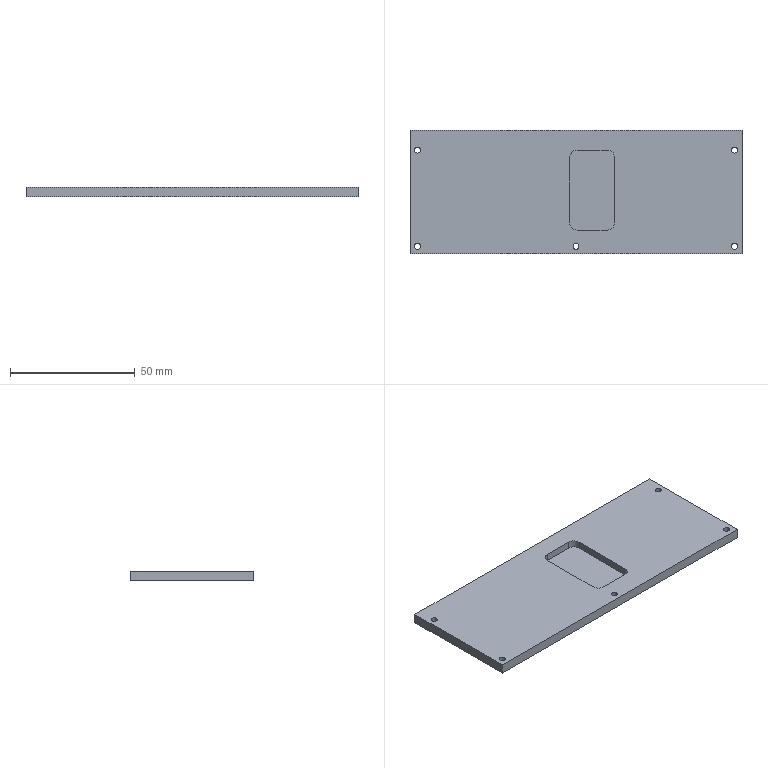Part | 1 solid | 48 faces | box 133 x 49.5 x 4 mm | volume 24425 mm3 | cylinder 28 | plane 16 | cone 4 | commonest cylinder face diameters 2.4 x10 4 x10 1.6 x4 6 x4
STEP:
#1=CARTESIAN_POINT('',(31.5,19.55,-2.8));
#2=VERTEX_POINT('',#1);
#3=CARTESIAN_POINT('',(31.5,19.55,-1.2));
#4=VERTEX_POINT('',#3);
#5=CARTESIAN_POINT('',(31.5,19.55,-2.));
#6=DIRECTION('',(0.,1.,0.));
#7=DIRECTION('',(0.,0.,1.));
#8=AXIS2_PLACEMENT_3D('',#5,#6,#7);
#9=CIRCLE('',#8,0.8);
#10=EDGE_CURVE('',#2,#4,#9,.T.);
#11=ORIENTED_EDGE('',*,*,#10,.F.);
#12=CARTESIAN_POINT('',(31.5,24.75,-2.8));
#13=VERTEX_POINT('',#12);
#14=CARTESIAN_POINT('',(31.5,24.75,-2.8));
#15=DIRECTION('',(0.,1.,0.));
#16=VECTOR('',#15,1000.);
#17=LINE('',#14,#16);
#18=EDGE_CURVE('',#2,#13,#17,.T.);
#19=ORIENTED_EDGE('',*,*,#18,.T.);
#20=CARTESIAN_POINT('',(31.5,24.75,-1.2));
#21=VERTEX_POINT('',#20);
#22=CARTESIAN_POINT('',(31.5,24.75,-2.));
#23=DIRECTION('',(0.,1.,0.));
#24=DIRECTION('',(0.,0.,1.));
#25=AXIS2_PLACEMENT_3D('',#22,#23,#24);
#26=CIRCLE('',#25,0.8);
#27=EDGE_CURVE('',#13,#21,#26,.T.);
#28=ORIENTED_EDGE('',*,*,#27,.T.);
#29=CARTESIAN_POINT('',(31.5,24.75,-1.2));
#30=DIRECTION('',(0.,1.,0.));
#31=VECTOR('',#30,1000.);
#32=LINE('',#29,#31);
#33=EDGE_CURVE('',#4,#21,#32,.T.);
#34=ORIENTED_EDGE('',*,*,#33,.F.);
#35=EDGE_LOOP('',(#11,#19,#28,#34));
#36=FACE_BOUND('',#35,.T.);
#37=CARTESIAN_POINT('',(31.5,24.75,-2.));
#38=DIRECTION('',(0.,1.,0.));
#39=DIRECTION('',(0.,0.,-1.));
#40=AXIS2_PLACEMENT_3D('',#37,#38,#39);
#41=CYLINDRICAL_SURFACE('',#40,0.8);
#42=ADVANCED_FACE('',(#36),#41,.F.);
#43=CARTESIAN_POINT('',(31.5,19.069,-2.));
#44=VERTEX_POINT('',#43);
#45=CARTESIAN_POINT('',(31.5,19.55,-1.2));
#46=DIRECTION('',(0.,0.515,0.8572));
#47=VECTOR('',#46,1000.);
#48=LINE('',#45,#47);
#49=EDGE_CURVE('',#44,#4,#48,.T.);
#50=ORIENTED_EDGE('',*,*,#49,.F.);
#51=CARTESIAN_POINT('',(31.5,19.55,-2.8));
#52=DIRECTION('',(0.,0.515,-0.8572));
#53=VECTOR('',#52,1000.);
#54=LINE('',#51,#53);
#55=EDGE_CURVE('',#44,#2,#54,.T.);
#56=ORIENTED_EDGE('',*,*,#55,.T.);
#57=ORIENTED_EDGE('',*,*,#10,.T.);
#58=EDGE_LOOP('',(#50,#56,#57));
#59=FACE_BOUND('',#58,.T.);
#60=CARTESIAN_POINT('',(31.5,19.55,-2.));
#61=DIRECTION('',(0.,1.,0.));
#62=DIRECTION('',(0.,0.,-1.));
#63=AXIS2_PLACEMENT_3D('',#60,#61,#62);
#64=CONICAL_SURFACE('',#63,0.8,1.03);
#65=ADVANCED_FACE('',(#59),#64,.F.);
#66=CARTESIAN_POINT('',(-31.5,19.55,-2.8));
#67=VERTEX_POINT('',#66);
#68=CARTESIAN_POINT('',(-31.5,19.55,-1.2));
#69=VERTEX_POINT('',#68);
#70=CARTESIAN_POINT('',(-31.5,19.55,-2.));
#71=DIRECTION('',(0.,1.,0.));
#72=DIRECTION('',(0.,0.,1.));
#73=AXIS2_PLACEMENT_3D('',#70,#71,#72);
#74=CIRCLE('',#73,0.8);
#75=EDGE_CURVE('',#67,#69,#74,.T.);
#76=ORIENTED_EDGE('',*,*,#75,.F.);
#77=CARTESIAN_POINT('',(-31.5,24.75,-2.8));
#78=VERTEX_POINT('',#77);
#79=CARTESIAN_POINT('',(-31.5,24.75,-2.8));
#80=DIRECTION('',(0.,1.,0.));
#81=VECTOR('',#80,1000.);
#82=LINE('',#79,#81);
#83=EDGE_CURVE('',#67,#78,#82,.T.);
#84=ORIENTED_EDGE('',*,*,#83,.T.);
#85=CARTESIAN_POINT('',(-31.5,24.75,-1.2));
#86=VERTEX_POINT('',#85);
#87=CARTESIAN_POINT('',(-31.5,24.75,-2.));
#88=DIRECTION('',(0.,1.,0.));
#89=DIRECTION('',(0.,0.,1.));
#90=AXIS2_PLACEMENT_3D('',#87,#88,#89);
#91=CIRCLE('',#90,0.8);
#92=EDGE_CURVE('',#78,#86,#91,.T.);
#93=ORIENTED_EDGE('',*,*,#92,.T.);
#94=CARTESIAN_POINT('',(-31.5,24.75,-1.2));
#95=DIRECTION('',(0.,1.,0.));
#96=VECTOR('',#95,1000.);
#97=LINE('',#94,#96);
#98=EDGE_CURVE('',#69,#86,#97,.T.);
#99=ORIENTED_EDGE('',*,*,#98,.F.);
#100=EDGE_LOOP('',(#76,#84,#93,#99));
#101=FACE_BOUND('',#100,.T.);
#102=CARTESIAN_POINT('',(-31.5,24.75,-2.));
#103=DIRECTION('',(0.,1.,0.));
#104=DIRECTION('',(0.,0.,-1.));
#105=AXIS2_PLACEMENT_3D('',#102,#103,#104);
#106=CYLINDRICAL_SURFACE('',#105,0.8);
#107=ADVANCED_FACE('',(#101),#106,.F.);
#108=CARTESIAN_POINT('',(-31.5,19.069,-2.));
#109=VERTEX_POINT('',#108);
#110=CARTESIAN_POINT('',(-31.5,19.55,-1.2));
#111=DIRECTION('',(0.,0.515,0.8572));
#112=VECTOR('',#111,1000.);
#113=LINE('',#110,#112);
#114=EDGE_CURVE('',#109,#69,#113,.T.);
#115=ORIENTED_EDGE('',*,*,#114,.F.);
#116=CARTESIAN_POINT('',(-31.5,19.55,-2.8));
#117=DIRECTION('',(0.,0.515,-0.8572));
#118=VECTOR('',#117,1000.);
#119=LINE('',#116,#118);
#120=EDGE_CURVE('',#109,#67,#119,.T.);
#121=ORIENTED_EDGE('',*,*,#120,.T.);
#122=ORIENTED_EDGE('',*,*,#75,.T.);
#123=EDGE_LOOP('',(#115,#121,#122));
#124=FACE_BOUND('',#123,.T.);
#125=CARTESIAN_POINT('',(-31.5,19.55,-2.));
#126=DIRECTION('',(0.,1.,0.));
#127=DIRECTION('',(0.,0.,-1.));
#128=AXIS2_PLACEMENT_3D('',#125,#126,#127);
#129=CONICAL_SURFACE('',#128,0.8,1.03);
#130=ADVANCED_FACE('',(#124),#129,.F.);
#131=CARTESIAN_POINT('',(-61.5,16.75,-1.7));
#132=VERTEX_POINT('',#131);
#133=CARTESIAN_POINT('',(-65.5,16.75,-1.7));
#134=VERTEX_POINT('',#133);
#135=CARTESIAN_POINT('',(-63.5,16.75,-1.7));
#136=DIRECTION('',(0.,0.,-1.));
#137=DIRECTION('',(-1.,0.,0.));
#138=AXIS2_PLACEMENT_3D('',#135,#136,#137);
#139=CIRCLE('',#138,2.);
#140=EDGE_CURVE('',#132,#134,#139,.T.);
#141=ORIENTED_EDGE('',*,*,#140,.F.);
#142=CARTESIAN_POINT('',(-61.5,16.75,-4.));
#143=VERTEX_POINT('',#142);
#144=CARTESIAN_POINT('',(-61.5,16.75,-4.));
#145=DIRECTION('',(0.,0.,-1.));
#146=VECTOR('',#145,1000.);
#147=LINE('',#144,#146);
#148=EDGE_CURVE('',#132,#143,#147,.T.);
#149=ORIENTED_EDGE('',*,*,#148,.T.);
#150=CARTESIAN_POINT('',(-65.5,16.75,-4.));
#151=VERTEX_POINT('',#150);
#152=CARTESIAN_POINT('',(-63.5,16.75,-4.));
#153=DIRECTION('',(0.,0.,-1.));
#154=DIRECTION('',(-1.,0.,0.));
#155=AXIS2_PLACEMENT_3D('',#152,#153,#154);
#156=CIRCLE('',#155,2.);
#157=EDGE_CURVE('',#143,#151,#156,.T.);
#158=ORIENTED_EDGE('',*,*,#157,.T.);
#159=CARTESIAN_POINT('',(-65.5,16.75,-4.));
#160=DIRECTION('',(0.,0.,-1.));
#161=VECTOR('',#160,1000.);
#162=LINE('',#159,#161);
#163=EDGE_CURVE('',#134,#151,#162,.T.);
#164=ORIENTED_EDGE('',*,*,#163,.F.);
#165=EDGE_LOOP('',(#141,#149,#158,#164));
#166=FACE_BOUND('',#165,.T.);
#167=CARTESIAN_POINT('',(-63.5,16.75,-4.));
#168=DIRECTION('',(0.,0.,-1.));
#169=DIRECTION('',(1.,0.,0.));
#170=AXIS2_PLACEMENT_3D('',#167,#168,#169);
#171=CYLINDRICAL_SURFACE('',#170,2.);
#172=ADVANCED_FACE('',(#166),#171,.F.);
#173=CARTESIAN_POINT('',(-64.7,16.75,0.));
#174=VERTEX_POINT('',#173);
#175=CARTESIAN_POINT('',(-62.3,16.75,0.));
#176=VERTEX_POINT('',#175);
#177=CARTESIAN_POINT('',(-63.5,16.75,0.));
#178=DIRECTION('',(0.,0.,1.));
#179=DIRECTION('',(1.,0.,0.));
#180=AXIS2_PLACEMENT_3D('',#177,#178,#179);
#181=CIRCLE('',#180,1.2);
#182=EDGE_CURVE('',#174,#176,#181,.T.);
#183=ORIENTED_EDGE('',*,*,#182,.T.);
#184=CARTESIAN_POINT('',(-62.3,16.75,-1.7));
#185=VERTEX_POINT('',#184);
#186=CARTESIAN_POINT('',(-62.3,16.75,-4.));
#187=DIRECTION('',(0.,0.,-1.));
#188=VECTOR('',#187,1000.);
#189=LINE('',#186,#188);
#190=EDGE_CURVE('',#176,#185,#189,.T.);
#191=ORIENTED_EDGE('',*,*,#190,.T.);
#192=CARTESIAN_POINT('',(-64.7,16.75,-1.7));
#193=VERTEX_POINT('',#192);
#194=CARTESIAN_POINT('',(-63.5,16.75,-1.7));
#195=DIRECTION('',(0.,0.,-1.));
#196=DIRECTION('',(-1.,0.,0.));
#197=AXIS2_PLACEMENT_3D('',#194,#195,#196);
#198=CIRCLE('',#197,1.2);
#199=EDGE_CURVE('',#185,#193,#198,.T.);
#200=ORIENTED_EDGE('',*,*,#199,.T.);
#201=CARTESIAN_POINT('',(-64.7,16.75,-4.));
#202=DIRECTION('',(0.,0.,-1.));
#203=VECTOR('',#202,1000.);
#204=LINE('',#201,#203);
#205=EDGE_CURVE('',#174,#193,#204,.T.);
#206=ORIENTED_EDGE('',*,*,#205,.F.);
#207=EDGE_LOOP('',(#183,#191,#200,#206));
#208=FACE_BOUND('',#207,.T.);
#209=CARTESIAN_POINT('',(-63.5,16.75,-4.));
#210=DIRECTION('',(0.,0.,-1.));
#211=DIRECTION('',(1.,0.,0.));
#212=AXIS2_PLACEMENT_3D('',#209,#210,#211);
#213=CYLINDRICAL_SURFACE('',#212,1.2);
#214=ADVANCED_FACE('',(#208),#213,.F.);
#215=CARTESIAN_POINT('',(-61.5,-21.75,-1.7));
#216=VERTEX_POINT('',#215);
#217=CARTESIAN_POINT('',(-65.5,-21.75,-1.7));
#218=VERTEX_POINT('',#217);
#219=CARTESIAN_POINT('',(-63.5,-21.75,-1.7));
#220=DIRECTION('',(0.,0.,-1.));
#221=DIRECTION('',(-1.,0.,0.));
#222=AXIS2_PLACEMENT_3D('',#219,#220,#221);
#223=CIRCLE('',#222,2.);
#224=EDGE_CURVE('',#216,#218,#223,.T.);
#225=ORIENTED_EDGE('',*,*,#224,.F.);
#226=CARTESIAN_POINT('',(-61.5,-21.75,-4.));
#227=VERTEX_POINT('',#226);
#228=CARTESIAN_POINT('',(-61.5,-21.75,-4.));
#229=DIRECTION('',(0.,0.,-1.));
#230=VECTOR('',#229,1000.);
#231=LINE('',#228,#230);
#232=EDGE_CURVE('',#216,#227,#231,.T.);
#233=ORIENTED_EDGE('',*,*,#232,.T.);
#234=CARTESIAN_POINT('',(-65.5,-21.75,-4.));
#235=VERTEX_POINT('',#234);
#236=CARTESIAN_POINT('',(-63.5,-21.75,-4.));
#237=DIRECTION('',(0.,0.,-1.));
#238=DIRECTION('',(-1.,0.,0.));
#239=AXIS2_PLACEMENT_3D('',#236,#237,#238);
#240=CIRCLE('',#239,2.);
#241=EDGE_CURVE('',#227,#235,#240,.T.);
#242=ORIENTED_EDGE('',*,*,#241,.T.);
#243=CARTESIAN_POINT('',(-65.5,-21.75,-4.));
#244=DIRECTION('',(0.,0.,-1.));
#245=VECTOR('',#244,1000.);
#246=LINE('',#243,#245);
#247=EDGE_CURVE('',#218,#235,#246,.T.);
#248=ORIENTED_EDGE('',*,*,#247,.F.);
#249=EDGE_LOOP('',(#225,#233,#242,#248));
#250=FACE_BOUND('',#249,.T.);
#251=CARTESIAN_POINT('',(-63.5,-21.75,-4.));
#252=DIRECTION('',(0.,0.,-1.));
#253=DIRECTION('',(1.,0.,0.));
#254=AXIS2_PLACEMENT_3D('',#251,#252,#253);
#255=CYLINDRICAL_SURFACE('',#254,2.);
#256=ADVANCED_FACE('',(#250),#255,.F.);
#257=CARTESIAN_POINT('',(-64.7,-21.75,0.));
#258=VERTEX_POINT('',#257);
#259=CARTESIAN_POINT('',(-62.3,-21.75,0.));
#260=VERTEX_POINT('',#259);
#261=CARTESIAN_POINT('',(-63.5,-21.75,0.));
#262=DIRECTION('',(0.,0.,1.));
#263=DIRECTION('',(1.,0.,0.));
#264=AXIS2_PLACEMENT_3D('',#261,#262,#263);
#265=CIRCLE('',#264,1.2);
#266=EDGE_CURVE('',#258,#260,#265,.T.);
#267=ORIENTED_EDGE('',*,*,#266,.T.);
#268=CARTESIAN_POINT('',(-62.3,-21.75,-1.7));
#269=VERTEX_POINT('',#268);
#270=CARTESIAN_POINT('',(-62.3,-21.75,-4.));
#271=DIRECTION('',(0.,0.,-1.));
#272=VECTOR('',#271,1000.);
#273=LINE('',#270,#272);
#274=EDGE_CURVE('',#260,#269,#273,.T.);
#275=ORIENTED_EDGE('',*,*,#274,.T.);
#276=CARTESIAN_POINT('',(-64.7,-21.75,-1.7));
#277=VERTEX_POINT('',#276);
#278=CARTESIAN_POINT('',(-63.5,-21.75,-1.7));
#279=DIRECTION('',(0.,0.,-1.));
#280=DIRECTION('',(-1.,0.,0.));
#281=AXIS2_PLACEMENT_3D('',#278,#279,#280);
#282=CIRCLE('',#281,1.2);
#283=EDGE_CURVE('',#269,#277,#282,.T.);
#284=ORIENTED_EDGE('',*,*,#283,.T.);
#285=CARTESIAN_POINT('',(-64.7,-21.75,-4.));
#286=DIRECTION('',(0.,0.,-1.));
#287=VECTOR('',#286,1000.);
#288=LINE('',#285,#287);
#289=EDGE_CURVE('',#258,#277,#288,.T.);
#290=ORIENTED_EDGE('',*,*,#289,.F.);
#291=EDGE_LOOP('',(#267,#275,#284,#290));
#292=FACE_BOUND('',#291,.T.);
#293=CARTESIAN_POINT('',(-63.5,-21.75,-4.));
#294=DIRECTION('',(0.,0.,-1.));
#295=DIRECTION('',(1.,0.,0.));
#296=AXIS2_PLACEMENT_3D('',#293,#294,#295);
#297=CYLINDRICAL_SURFACE('',#296,1.2);
#298=ADVANCED_FACE('',(#292),#297,.F.);
#299=CARTESIAN_POINT('',(2.,-21.75,-1.7));
#300=VERTEX_POINT('',#299);
#301=CARTESIAN_POINT('',(-2.,-21.75,-1.7));
#302=VERTEX_POINT('',#301);
#303=CARTESIAN_POINT('',(0.,-21.75,-1.7));
#304=DIRECTION('',(0.,0.,-1.));
#305=DIRECTION('',(-1.,0.,0.));
#306=AXIS2_PLACEMENT_3D('',#303,#304,#305);
#307=CIRCLE('',#306,2.);
#308=EDGE_CURVE('',#300,#302,#307,.T.);
#309=ORIENTED_EDGE('',*,*,#308,.F.);
#310=CARTESIAN_POINT('',(2.,-21.75,-4.));
#311=VERTEX_POINT('',#310);
#312=CARTESIAN_POINT('',(2.,-21.75,-4.));
#313=DIRECTION('',(0.,0.,-1.));
#314=VECTOR('',#313,1000.);
#315=LINE('',#312,#314);
#316=EDGE_CURVE('',#300,#311,#315,.T.);
#317=ORIENTED_EDGE('',*,*,#316,.T.);
#318=CARTESIAN_POINT('',(-2.,-21.75,-4.));
#319=VERTEX_POINT('',#318);
#320=CARTESIAN_POINT('',(0.,-21.75,-4.));
#321=DIRECTION('',(0.,0.,-1.));
#322=DIRECTION('',(-1.,0.,0.));
#323=AXIS2_PLACEMENT_3D('',#320,#321,#322);
#324=CIRCLE('',#323,2.);
#325=EDGE_CURVE('',#311,#319,#324,.T.);
#326=ORIENTED_EDGE('',*,*,#325,.T.);
#327=CARTESIAN_POINT('',(-2.,-21.75,-4.));
#328=DIRECTION('',(0.,0.,-1.));
#329=VECTOR('',#328,1000.);
#330=LINE('',#327,#329);
#331=EDGE_CURVE('',#302,#319,#330,.T.);
#332=ORIENTED_EDGE('',*,*,#331,.F.);
#333=EDGE_LOOP('',(#309,#317,#326,#332));
#334=FACE_BOUND('',#333,.T.);
#335=CARTESIAN_POINT('',(0.,-21.75,-4.));
#336=DIRECTION('',(0.,0.,-1.));
#337=DIRECTION('',(1.,0.,0.));
#338=AXIS2_PLACEMENT_3D('',#335,#336,#337);
#339=CYLINDRICAL_SURFACE('',#338,2.);
#340=ADVANCED_FACE('',(#334),#339,.F.);
#341=CARTESIAN_POINT('',(-1.2,-21.75,0.));
#342=VERTEX_POINT('',#341);
#343=CARTESIAN_POINT('',(1.2,-21.75,0.));
#344=VERTEX_POINT('',#343);
#345=CARTESIAN_POINT('',(0.,-21.75,0.));
#346=DIRECTION('',(0.,0.,1.));
#347=DIRECTION('',(1.,0.,0.));
#348=AXIS2_PLACEMENT_3D('',#345,#346,#347);
#349=CIRCLE('',#348,1.2);
#350=EDGE_CURVE('',#342,#344,#349,.T.);
#351=ORIENTED_EDGE('',*,*,#350,.T.);
#352=CARTESIAN_POINT('',(1.2,-21.75,-1.7));
#353=VERTEX_POINT('',#352);
#354=CARTESIAN_POINT('',(1.2,-21.75,-4.));
#355=DIRECTION('',(0.,0.,-1.));
#356=VECTOR('',#355,1000.);
#357=LINE('',#354,#356);
#358=EDGE_CURVE('',#344,#353,#357,.T.);
#359=ORIENTED_EDGE('',*,*,#358,.T.);
#360=CARTESIAN_POINT('',(-1.2,-21.75,-1.7));
#361=VERTEX_POINT('',#360);
#362=CARTESIAN_POINT('',(0.,-21.75,-1.7));
#363=DIRECTION('',(0.,0.,-1.));
#364=DIRECTION('',(-1.,0.,0.));
#365=AXIS2_PLACEMENT_3D('',#362,#363,#364);
#366=CIRCLE('',#365,1.2);
#367=EDGE_CURVE('',#353,#361,#366,.T.);
#368=ORIENTED_EDGE('',*,*,#367,.T.);
#369=CARTESIAN_POINT('',(-1.2,-21.75,-4.));
#370=DIRECTION('',(0.,0.,-1.));
#371=VECTOR('',#370,1000.);
#372=LINE('',#369,#371);
#373=EDGE_CURVE('',#342,#361,#372,.T.);
#374=ORIENTED_EDGE('',*,*,#373,.F.);
#375=EDGE_LOOP('',(#351,#359,#368,#374));
#376=FACE_BOUND('',#375,.T.);
#377=CARTESIAN_POINT('',(0.,-21.75,-4.));
#378=DIRECTION('',(0.,0.,-1.));
#379=DIRECTION('',(1.,0.,0.));
#380=AXIS2_PLACEMENT_3D('',#377,#378,#379);
#381=CYLINDRICAL_SURFACE('',#380,1.2);
#382=ADVANCED_FACE('',(#376),#381,.F.);
#383=CARTESIAN_POINT('',(65.5,-21.75,-1.7));
#384=VERTEX_POINT('',#383);
#385=CARTESIAN_POINT('',(61.5,-21.75,-1.7));
#386=VERTEX_POINT('',#385);
#387=CARTESIAN_POINT('',(63.5,-21.75,-1.7));
#388=DIRECTION('',(0.,0.,-1.));
#389=DIRECTION('',(-1.,0.,0.));
#390=AXIS2_PLACEMENT_3D('',#387,#388,#389);
#391=CIRCLE('',#390,2.);
#392=EDGE_CURVE('',#384,#386,#391,.T.);
#393=ORIENTED_EDGE('',*,*,#392,.F.);
#394=CARTESIAN_POINT('',(65.5,-21.75,-4.));
#395=VERTEX_POINT('',#394);
#396=CARTESIAN_POINT('',(65.5,-21.75,-4.));
#397=DIRECTION('',(0.,0.,-1.));
#398=VECTOR('',#397,1000.);
#399=LINE('',#396,#398);
#400=EDGE_CURVE('',#384,#395,#399,.T.);
#401=ORIENTED_EDGE('',*,*,#400,.T.);
#402=CARTESIAN_POINT('',(61.5,-21.75,-4.));
#403=VERTEX_POINT('',#402);
#404=CARTESIAN_POINT('',(63.5,-21.75,-4.));
#405=DIRECTION('',(0.,0.,-1.));
#406=DIRECTION('',(-1.,0.,0.));
#407=AXIS2_PLACEMENT_3D('',#404,#405,#406);
#408=CIRCLE('',#407,2.);
#409=EDGE_CURVE('',#395,#403,#408,.T.);
#410=ORIENTED_EDGE('',*,*,#409,.T.);
#411=CARTESIAN_POINT('',(61.5,-21.75,-4.));
#412=DIRECTION('',(0.,0.,-1.));
#413=VECTOR('',#412,1000.);
#414=LINE('',#411,#413);
#415=EDGE_CURVE('',#386,#403,#414,.T.);
#416=ORIENTED_EDGE('',*,*,#415,.F.);
#417=EDGE_LOOP('',(#393,#401,#410,#416));
#418=FACE_BOUND('',#417,.T.);
#419=CARTESIAN_POINT('',(63.5,-21.75,-4.));
#420=DIRECTION('',(0.,0.,-1.));
#421=DIRECTION('',(1.,0.,0.));
#422=AXIS2_PLACEMENT_3D('',#419,#420,#421);
#423=CYLINDRICAL_SURFACE('',#422,2.);
#424=ADVANCED_FACE('',(#418),#423,.F.);
#425=CARTESIAN_POINT('',(62.3,-21.75,0.));
#426=VERTEX_POINT('',#425);
#427=CARTESIAN_POINT('',(64.7,-21.75,0.));
#428=VERTEX_POINT('',#427);
#429=CARTESIAN_POINT('',(63.5,-21.75,0.));
#430=DIRECTION('',(0.,0.,1.));
#431=DIRECTION('',(1.,0.,0.));
#432=AXIS2_PLACEMENT_3D('',#429,#430,#431);
#433=CIRCLE('',#432,1.2);
#434=EDGE_CURVE('',#426,#428,#433,.T.);
#435=ORIENTED_EDGE('',*,*,#434,.T.);
#436=CARTESIAN_POINT('',(64.7,-21.75,-1.7));
#437=VERTEX_POINT('',#436);
#438=CARTESIAN_POINT('',(64.7,-21.75,-4.));
#439=DIRECTION('',(0.,0.,-1.));
#440=VECTOR('',#439,1000.);
#441=LINE('',#438,#440);
#442=EDGE_CURVE('',#428,#437,#441,.T.);
#443=ORIENTED_EDGE('',*,*,#442,.T.);
#444=CARTESIAN_POINT('',(62.3,-21.75,-1.7));
#445=VERTEX_POINT('',#444);
#446=CARTESIAN_POINT('',(63.5,-21.75,-1.7));
#447=DIRECTION('',(0.,0.,-1.));
#448=DIRECTION('',(-1.,0.,0.));
#449=AXIS2_PLACEMENT_3D('',#446,#447,#448);
#450=CIRCLE('',#449,1.2);
#451=EDGE_CURVE('',#437,#445,#450,.T.);
#452=ORIENTED_EDGE('',*,*,#451,.T.);
#453=CARTESIAN_POINT('',(62.3,-21.75,-4.));
#454=DIRECTION('',(0.,0.,-1.));
#455=VECTOR('',#454,1000.);
#456=LINE('',#453,#455);
#457=EDGE_CURVE('',#426,#445,#456,.T.);
#458=ORIENTED_EDGE('',*,*,#457,.F.);
#459=EDGE_LOOP('',(#435,#443,#452,#458));
#460=FACE_BOUND('',#459,.T.);
#461=CARTESIAN_POINT('',(63.5,-21.75,-4.));
#462=DIRECTION('',(0.,0.,-1.));
#463=DIRECTION('',(1.,0.,0.));
#464=AXIS2_PLACEMENT_3D('',#461,#462,#463);
#465=CYLINDRICAL_SURFACE('',#464,1.2);
#466=ADVANCED_FACE('',(#460),#465,.F.);
#467=CARTESIAN_POINT('',(65.5,16.75,-1.7));
#468=VERTEX_POINT('',#467);
#469=CARTESIAN_POINT('',(61.5,16.75,-1.7));
#470=VERTEX_POINT('',#469);
#471=CARTESIAN_POINT('',(63.5,16.75,-1.7));
#472=DIRECTION('',(0.,0.,-1.));
#473=DIRECTION('',(-1.,0.,0.));
#474=AXIS2_PLACEMENT_3D('',#471,#472,#473);
#475=CIRCLE('',#474,2.);
#476=EDGE_CURVE('',#468,#470,#475,.T.);
#477=ORIENTED_EDGE('',*,*,#476,.F.);
#478=CARTESIAN_POINT('',(65.5,16.75,-4.));
#479=VERTEX_POINT('',#478);
#480=CARTESIAN_POINT('',(65.5,16.75,-4.));
#481=DIRECTION('',(0.,0.,-1.));
#482=VECTOR('',#481,1000.);
#483=LINE('',#480,#482);
#484=EDGE_CURVE('',#468,#479,#483,.T.);
#485=ORIENTED_EDGE('',*,*,#484,.T.);
#486=CARTESIAN_POINT('',(61.5,16.75,-4.));
#487=VERTEX_POINT('',#486);
#488=CARTESIAN_POINT('',(63.5,16.75,-4.));
#489=DIRECTION('',(0.,0.,-1.));
#490=DIRECTION('',(-1.,0.,0.));
#491=AXIS2_PLACEMENT_3D('',#488,#489,#490);
#492=CIRCLE('',#491,2.);
#493=EDGE_CURVE('',#479,#487,#492,.T.);
#494=ORIENTED_EDGE('',*,*,#493,.T.);
#495=CARTESIAN_POINT('',(61.5,16.75,-4.));
#496=DIRECTION('',(0.,0.,-1.));
#497=VECTOR('',#496,1000.);
#498=LINE('',#495,#497);
#499=EDGE_CURVE('',#470,#487,#498,.T.);
#500=ORIENTED_EDGE('',*,*,#499,.F.);
#501=EDGE_LOOP('',(#477,#485,#494,#500));
#502=FACE_BOUND('',#501,.T.);
#503=CARTESIAN_POINT('',(63.5,16.75,-4.));
#504=DIRECTION('',(0.,0.,-1.));
#505=DIRECTION('',(1.,0.,0.));
#506=AXIS2_PLACEMENT_3D('',#503,#504,#505);
#507=CYLINDRICAL_SURFACE('',#506,2.);
#508=ADVANCED_FACE('',(#502),#507,.F.);
#509=CARTESIAN_POINT('',(62.3,16.75,0.));
#510=VERTEX_POINT('',#509);
#511=CARTESIAN_POINT('',(64.7,16.75,0.));
#512=VERTEX_POINT('',#511);
#513=CARTESIAN_POINT('',(63.5,16.75,0.));
#514=DIRECTION('',(0.,0.,1.));
#515=DIRECTION('',(1.,0.,0.));
#516=AXIS2_PLACEMENT_3D('',#513,#514,#515);
#517=CIRCLE('',#516,1.2);
#518=EDGE_CURVE('',#510,#512,#517,.T.);
#519=ORIENTED_EDGE('',*,*,#518,.T.);
#520=CARTESIAN_POINT('',(64.7,16.75,-1.7));
#521=VERTEX_POINT('',#520);
#522=CARTESIAN_POINT('',(64.7,16.75,-4.));
#523=DIRECTION('',(0.,0.,-1.));
#524=VECTOR('',#523,1000.);
#525=LINE('',#522,#524);
#526=EDGE_CURVE('',#512,#521,#525,.T.);
#527=ORIENTED_EDGE('',*,*,#526,.T.);
#528=CARTESIAN_POINT('',(62.3,16.75,-1.7));
#529=VERTEX_POINT('',#528);
#530=CARTESIAN_POINT('',(63.5,16.75,-1.7));
#531=DIRECTION('',(0.,0.,-1.));
#532=DIRECTION('',(-1.,0.,0.));
#533=AXIS2_PLACEMENT_3D('',#530,#531,#532);
#534=CIRCLE('',#533,1.2);
#535=EDGE_CURVE('',#521,#529,#534,.T.);
#536=ORIENTED_EDGE('',*,*,#535,.T.);
#537=CARTESIAN_POINT('',(62.3,16.75,-4.));
#538=DIRECTION('',(0.,0.,-1.));
#539=VECTOR('',#538,1000.);
#540=LINE('',#537,#539);
#541=EDGE_CURVE('',#510,#529,#540,.T.);
#542=ORIENTED_EDGE('',*,*,#541,.F.);
#543=EDGE_LOOP('',(#519,#527,#536,#542));
#544=FACE_BOUND('',#543,.T.);
#545=CARTESIAN_POINT('',(63.5,16.75,-4.));
#546=DIRECTION('',(0.,0.,-1.));
#547=DIRECTION('',(1.,0.,0.));
#548=AXIS2_PLACEMENT_3D('',#545,#546,#547);
#549=CYLINDRICAL_SURFACE('',#548,1.2);
#550=ADVANCED_FACE('',(#544),#549,.F.);
#551=CARTESIAN_POINT('',(66.5,-24.75,-4.));
#552=VERTEX_POINT('',#551);
#553=CARTESIAN_POINT('',(66.5,24.75,-4.));
#554=VERTEX_POINT('',#553);
#555=CARTESIAN_POINT('',(66.5,24.75,-4.));
#556=DIRECTION('',(0.,1.,0.));
#557=VECTOR('',#556,1000.);
#558=LINE('',#555,#557);
#559=EDGE_CURVE('',#552,#554,#558,.T.);
#560=ORIENTED_EDGE('',*,*,#559,.T.);
#561=CARTESIAN_POINT('',(66.5,24.75,0.));
#562=VERTEX_POINT('',#561);
#563=CARTESIAN_POINT('',(66.5,24.75,0.));
#564=DIRECTION('',(0.,0.,-1.));
#565=VECTOR('',#564,1000.);
#566=LINE('',#563,#565);
#567=EDGE_CURVE('',#562,#554,#566,.T.);
#568=ORIENTED_EDGE('',*,*,#567,.F.);
#569=CARTESIAN_POINT('',(66.5,-24.75,0.));
#570=VERTEX_POINT('',#569);
#571=CARTESIAN_POINT('',(66.5,24.75,0.));
#572=DIRECTION('',(0.,1.,0.));
#573=VECTOR('',#572,1000.);
#574=LINE('',#571,#573);
#575=EDGE_CURVE('',#570,#562,#574,.T.);
#576=ORIENTED_EDGE('',*,*,#575,.F.);
#577=CARTESIAN_POINT('',(66.5,-24.75,0.));
#578=DIRECTION('',(0.,0.,-1.));
#579=VECTOR('',#578,1000.);
#580=LINE('',#577,#579);
#581=EDGE_CURVE('',#570,#552,#580,.T.);
#582=ORIENTED_EDGE('',*,*,#581,.T.);
#583=EDGE_LOOP('',(#560,#568,#576,#582));
#584=FACE_BOUND('',#583,.T.);
#585=CARTESIAN_POINT('',(66.5,24.75,0.));
#586=DIRECTION('',(-1.,0.,0.));
#587=DIRECTION('',(0.,1.,0.));
#588=AXIS2_PLACEMENT_3D('',#585,#586,#587);
#589=PLANE('',#588);
#590=ADVANCED_FACE('',(#584),#589,.F.);
#591=CARTESIAN_POINT('',(31.5,24.75,-2.));
#592=DIRECTION('',(0.,1.,0.));
#593=DIRECTION('',(0.,0.,1.));
#594=AXIS2_PLACEMENT_3D('',#591,#592,#593);
#595=CIRCLE('',#594,0.8);
#596=EDGE_CURVE('',#21,#13,#595,.T.);
#597=ORIENTED_EDGE('',*,*,#596,.F.);
#598=ORIENTED_EDGE('',*,*,#27,.F.);
#599=EDGE_LOOP('',(#597,#598));
#600=FACE_BOUND('',#599,.T.);
#601=CARTESIAN_POINT('',(-31.5,24.75,-2.));
#602=DIRECTION('',(0.,1.,0.));
#603=DIRECTION('',(0.,0.,1.));
#604=AXIS2_PLACEMENT_3D('',#601,#602,#603);
#605=CIRCLE('',#604,0.8);
#606=EDGE_CURVE('',#86,#78,#605,.T.);
#607=ORIENTED_EDGE('',*,*,#606,.F.);
#608=ORIENTED_EDGE('',*,*,#92,.F.);
#609=EDGE_LOOP('',(#607,#608));
#610=FACE_BOUND('',#609,.T.);
#611=CARTESIAN_POINT('',(-66.5,24.75,-4.));
#612=VERTEX_POINT('',#611);
#613=CARTESIAN_POINT('',(-66.5,24.75,-4.));
#614=DIRECTION('',(-1.,0.,0.));
#615=VECTOR('',#614,1000.);
#616=LINE('',#613,#615);
#617=EDGE_CURVE('',#554,#612,#616,.T.);
#618=ORIENTED_EDGE('',*,*,#617,.T.);
#619=CARTESIAN_POINT('',(-66.5,24.75,0.));
#620=VERTEX_POINT('',#619);
#621=CARTESIAN_POINT('',(-66.5,24.75,0.));
#622=DIRECTION('',(0.,0.,-1.));
#623=VECTOR('',#622,1000.);
#624=LINE('',#621,#623);
#625=EDGE_CURVE('',#620,#612,#624,.T.);
#626=ORIENTED_EDGE('',*,*,#625,.F.);
#627=CARTESIAN_POINT('',(-66.5,24.75,0.));
#628=DIRECTION('',(-1.,0.,0.));
#629=VECTOR('',#628,1000.);
#630=LINE('',#627,#629);
#631=EDGE_CURVE('',#562,#620,#630,.T.);
#632=ORIENTED_EDGE('',*,*,#631,.F.);
#633=ORIENTED_EDGE('',*,*,#567,.T.);
#634=EDGE_LOOP('',(#618,#626,#632,#633));
#635=FACE_BOUND('',#634,.T.);
#636=CARTESIAN_POINT('',(-66.5,24.75,0.));
#637=DIRECTION('',(0.,-1.,0.));
#638=DIRECTION('',(0.,0.,1.));
#639=AXIS2_PLACEMENT_3D('',#636,#637,#638);
#640=PLANE('',#639);
#641=ADVANCED_FACE('',(#600,#610,#635),#640,.F.);
#642=CARTESIAN_POINT('',(-66.5,-24.75,-4.));
#643=VERTEX_POINT('',#642);
#644=CARTESIAN_POINT('',(-66.5,24.75,-4.));
#645=DIRECTION('',(0.,-1.,0.));
#646=VECTOR('',#645,1000.);
#647=LINE('',#644,#646);
#648=EDGE_CURVE('',#612,#643,#647,.T.);
#649=ORIENTED_EDGE('',*,*,#648,.T.);
#650=CARTESIAN_POINT('',(-66.5,-24.75,0.));
#651=VERTEX_POINT('',#650);
#652=CARTESIAN_POINT('',(-66.5,-24.75,0.));
#653=DIRECTION('',(0.,0.,-1.));
#654=VECTOR('',#653,1000.);
#655=LINE('',#652,#654);
#656=EDGE_CURVE('',#651,#643,#655,.T.);
#657=ORIENTED_EDGE('',*,*,#656,.F.);
#658=CARTESIAN_POINT('',(-66.5,24.75,0.));
#659=DIRECTION('',(0.,-1.,0.));
#660=VECTOR('',#659,1000.);
#661=LINE('',#658,#660);
#662=EDGE_CURVE('',#620,#651,#661,.T.);
#663=ORIENTED_EDGE('',*,*,#662,.F.);
#664=ORIENTED_EDGE('',*,*,#625,.T.);
#665=EDGE_LOOP('',(#649,#657,#663,#664));
#666=FACE_BOUND('',#665,.T.);
#667=CARTESIAN_POINT('',(-66.5,24.75,0.));
#668=DIRECTION('',(1.,0.,0.));
#669=DIRECTION('',(0.,0.,1.));
#670=AXIS2_PLACEMENT_3D('',#667,#668,#669);
#671=PLANE('',#670);
#672=ADVANCED_FACE('',(#666),#671,.F.);
#673=CARTESIAN_POINT('',(-66.5,-24.75,-4.));
#674=DIRECTION('',(1.,0.,0.));
#675=VECTOR('',#674,1000.);
#676=LINE('',#673,#675);
#677=EDGE_CURVE('',#643,#552,#676,.T.);
#678=ORIENTED_EDGE('',*,*,#677,.T.);
#679=ORIENTED_EDGE('',*,*,#581,.F.);
#680=CARTESIAN_POINT('',(-66.5,-24.75,0.));
#681=DIRECTION('',(1.,0.,0.));
#682=VECTOR('',#681,1000.);
#683=LINE('',#680,#682);
#684=EDGE_CURVE('',#651,#570,#683,.T.);
#685=ORIENTED_EDGE('',*,*,#684,.F.);
#686=ORIENTED_EDGE('',*,*,#656,.T.);
#687=EDGE_LOOP('',(#678,#679,#685,#686));
#688=FACE_BOUND('',#687,.T.);
#689=CARTESIAN_POINT('',(-66.5,-24.75,0.));
#690=DIRECTION('',(0.,1.,0.));
#691=DIRECTION('',(0.,0.,-1.));
#692=AXIS2_PLACEMENT_3D('',#689,#690,#691);
#693=PLANE('',#692);
#694=ADVANCED_FACE('',(#688),#693,.F.);
#695=CARTESIAN_POINT('',(15.5,-12.25,0.));
#696=VERTEX_POINT('',#695);
#697=CARTESIAN_POINT('',(15.5,13.75,0.));
#698=VERTEX_POINT('',#697);
#699=CARTESIAN_POINT('',(15.5,16.75,0.));
#700=DIRECTION('',(0.,1.,0.));
#701=VECTOR('',#700,1000.);
#702=LINE('',#699,#701);
#703=EDGE_CURVE('',#696,#698,#702,.T.);
#704=ORIENTED_EDGE('',*,*,#703,.F.);
#705=CARTESIAN_POINT('',(12.5,-15.25,0.));
#706=VERTEX_POINT('',#705);
#707=CARTESIAN_POINT('',(12.5,-12.25,0.));
#708=DIRECTION('',(0.,0.,-1.));
#709=DIRECTION('',(1.,0.,0.));
#710=AXIS2_PLACEMENT_3D('',#707,#708,#709);
#711=CIRCLE('',#710,3.);
#712=EDGE_CURVE('',#696,#706,#711,.T.);
#713=ORIENTED_EDGE('',*,*,#712,.T.);
#714=CARTESIAN_POINT('',(0.5,-15.25,0.));
#715=VERTEX_POINT('',#714);
#716=CARTESIAN_POINT('',(-2.5,-15.25,0.));
#717=DIRECTION('',(1.,0.,0.));
#718=VECTOR('',#717,1000.);
#719=LINE('',#716,#718);
#720=EDGE_CURVE('',#715,#706,#719,.T.);
#721=ORIENTED_EDGE('',*,*,#720,.F.);
#722=CARTESIAN_POINT('',(-2.5,-12.25,0.));
#723=VERTEX_POINT('',#722);
#724=CARTESIAN_POINT('',(0.5,-12.25,0.));
#725=DIRECTION('',(0.,0.,-1.));
#726=DIRECTION('',(1.,0.,0.));
#727=AXIS2_PLACEMENT_3D('',#724,#725,#726);
#728=CIRCLE('',#727,3.);
#729=EDGE_CURVE('',#715,#723,#728,.T.);
#730=ORIENTED_EDGE('',*,*,#729,.T.);
#731=CARTESIAN_POINT('',(-2.5,13.75,0.));
#732=VERTEX_POINT('',#731);
#733=CARTESIAN_POINT('',(-2.5,16.75,0.));
#734=DIRECTION('',(0.,-1.,0.));
#735=VECTOR('',#734,1000.);
#736=LINE('',#733,#735);
#737=EDGE_CURVE('',#732,#723,#736,.T.);
#738=ORIENTED_EDGE('',*,*,#737,.F.);
#739=CARTESIAN_POINT('',(0.5,16.75,0.));
#740=VERTEX_POINT('',#739);
#741=CARTESIAN_POINT('',(0.5,13.75,0.));
#742=DIRECTION('',(0.,0.,-1.));
#743=DIRECTION('',(1.,0.,0.));
#744=AXIS2_PLACEMENT_3D('',#741,#742,#743);
#745=CIRCLE('',#744,3.);
#746=EDGE_CURVE('',#732,#740,#745,.T.);
#747=ORIENTED_EDGE('',*,*,#746,.T.);
#748=CARTESIAN_POINT('',(12.5,16.75,0.));
#749=VERTEX_POINT('',#748);
#750=CARTESIAN_POINT('',(-2.5,16.75,0.));
#751=DIRECTION('',(-1.,0.,0.));
#752=VECTOR('',#751,1000.);
#753=LINE('',#750,#752);
#754=EDGE_CURVE('',#749,#740,#753,.T.);
#755=ORIENTED_EDGE('',*,*,#754,.F.);
#756=CARTESIAN_POINT('',(12.5,13.75,0.));
#757=DIRECTION('',(0.,0.,-1.));
#758=DIRECTION('',(1.,0.,0.));
#759=AXIS2_PLACEMENT_3D('',#756,#757,#758);
#760=CIRCLE('',#759,3.);
#761=EDGE_CURVE('',#749,#698,#760,.T.);
#762=ORIENTED_EDGE('',*,*,#761,.T.);
#763=EDGE_LOOP('',(#704,#713,#721,#730,#738,#747,#755,#762));
#764=FACE_BOUND('',#763,.T.);
#765=ORIENTED_EDGE('',*,*,#182,.F.);
#766=CARTESIAN_POINT('',(-63.5,16.75,0.));
#767=DIRECTION('',(0.,0.,1.));
#768=DIRECTION('',(1.,0.,0.));
#769=AXIS2_PLACEMENT_3D('',#766,#767,#768);
#770=CIRCLE('',#769,1.2);
#771=EDGE_CURVE('',#176,#174,#770,.T.);
#772=ORIENTED_EDGE('',*,*,#771,.F.);
#773=EDGE_LOOP('',(#765,#772));
#774=FACE_BOUND('',#773,.T.);
#775=ORIENTED_EDGE('',*,*,#266,.F.);
#776=CARTESIAN_POINT('',(-63.5,-21.75,0.));
#777=DIRECTION('',(0.,0.,1.));
#778=DIRECTION('',(1.,0.,0.));
#779=AXIS2_PLACEMENT_3D('',#776,#777,#778);
#780=CIRCLE('',#779,1.2);
#781=EDGE_CURVE('',#260,#258,#780,.T.);
#782=ORIENTED_EDGE('',*,*,#781,.F.);
#783=EDGE_LOOP('',(#775,#782));
#784=FACE_BOUND('',#783,.T.);
#785=ORIENTED_EDGE('',*,*,#350,.F.);
#786=CARTESIAN_POINT('',(0.,-21.75,0.));
#787=DIRECTION('',(0.,0.,1.));
#788=DIRECTION('',(1.,0.,0.));
#789=AXIS2_PLACEMENT_3D('',#786,#787,#788);
#790=CIRCLE('',#789,1.2);
#791=EDGE_CURVE('',#344,#342,#790,.T.);
#792=ORIENTED_EDGE('',*,*,#791,.F.);
#793=EDGE_LOOP('',(#785,#792));
#794=FACE_BOUND('',#793,.T.);
#795=ORIENTED_EDGE('',*,*,#434,.F.);
#796=CARTESIAN_POINT('',(63.5,-21.75,0.));
#797=DIRECTION('',(0.,0.,1.));
#798=DIRECTION('',(1.,0.,0.));
#799=AXIS2_PLACEMENT_3D('',#796,#797,#798);
#800=CIRCLE('',#799,1.2);
#801=EDGE_CURVE('',#428,#426,#800,.T.);
#802=ORIENTED_EDGE('',*,*,#801,.F.);
#803=EDGE_LOOP('',(#795,#802));
#804=FACE_BOUND('',#803,.T.);
#805=ORIENTED_EDGE('',*,*,#518,.F.);
#806=CARTESIAN_POINT('',(63.5,16.75,0.));
#807=DIRECTION('',(0.,0.,1.));
#808=DIRECTION('',(1.,0.,0.));
#809=AXIS2_PLACEMENT_3D('',#806,#807,#808);
#810=CIRCLE('',#809,1.2);
#811=EDGE_CURVE('',#512,#510,#810,.T.);
#812=ORIENTED_EDGE('',*,*,#811,.F.);
#813=EDGE_LOOP('',(#805,#812));
#814=FACE_BOUND('',#813,.T.);
#815=ORIENTED_EDGE('',*,*,#575,.T.);
#816=ORIENTED_EDGE('',*,*,#631,.T.);
#817=ORIENTED_EDGE('',*,*,#662,.T.);
#818=ORIENTED_EDGE('',*,*,#684,.T.);
#819=EDGE_LOOP('',(#815,#816,#817,#818));
#820=FACE_BOUND('',#819,.T.);
#821=CARTESIAN_POINT('',(0.,0.,0.));
#822=DIRECTION('',(0.,0.,1.));
#823=DIRECTION('',(-1.,0.,0.));
#824=AXIS2_PLACEMENT_3D('',#821,#822,#823);
#825=PLANE('',#824);
#826=ADVANCED_FACE('',(#764,#774,#784,#794,#804,#814,#820),#825,.T.);
#827=CARTESIAN_POINT('',(-63.5,16.75,-4.));
#828=DIRECTION('',(0.,0.,-1.));
#829=DIRECTION('',(-1.,0.,0.));
#830=AXIS2_PLACEMENT_3D('',#827,#828,#829);
#831=CIRCLE('',#830,2.);
#832=EDGE_CURVE('',#151,#143,#831,.T.);
#833=ORIENTED_EDGE('',*,*,#832,.F.);
#834=ORIENTED_EDGE('',*,*,#157,.F.);
#835=EDGE_LOOP('',(#833,#834));
#836=FACE_BOUND('',#835,.T.);
#837=CARTESIAN_POINT('',(-63.5,-21.75,-4.));
#838=DIRECTION('',(0.,0.,-1.));
#839=DIRECTION('',(-1.,0.,0.));
#840=AXIS2_PLACEMENT_3D('',#837,#838,#839);
#841=CIRCLE('',#840,2.);
#842=EDGE_CURVE('',#235,#227,#841,.T.);
#843=ORIENTED_EDGE('',*,*,#842,.F.);
#844=ORIENTED_EDGE('',*,*,#241,.F.);
#845=EDGE_LOOP('',(#843,#844));
#846=FACE_BOUND('',#845,.T.);
#847=CARTESIAN_POINT('',(0.,-21.75,-4.));
#848=DIRECTION('',(0.,0.,-1.));
#849=DIRECTION('',(-1.,0.,0.));
#850=AXIS2_PLACEMENT_3D('',#847,#848,#849);
#851=CIRCLE('',#850,2.);
#852=EDGE_CURVE('',#319,#311,#851,.T.);
#853=ORIENTED_EDGE('',*,*,#852,.F.);
#854=ORIENTED_EDGE('',*,*,#325,.F.);
#855=EDGE_LOOP('',(#853,#854));
#856=FACE_BOUND('',#855,.T.);
#857=CARTESIAN_POINT('',(63.5,-21.75,-4.));
#858=DIRECTION('',(0.,0.,-1.));
#859=DIRECTION('',(-1.,0.,0.));
#860=AXIS2_PLACEMENT_3D('',#857,#858,#859);
#861=CIRCLE('',#860,2.);
#862=EDGE_CURVE('',#403,#395,#861,.T.);
#863=ORIENTED_EDGE('',*,*,#862,.F.);
#864=ORIENTED_EDGE('',*,*,#409,.F.);
#865=EDGE_LOOP('',(#863,#864));
#866=FACE_BOUND('',#865,.T.);
#867=CARTESIAN_POINT('',(63.5,16.75,-4.));
#868=DIRECTION('',(0.,0.,-1.));
#869=DIRECTION('',(-1.,0.,0.));
#870=AXIS2_PLACEMENT_3D('',#867,#868,#869);
#871=CIRCLE('',#870,2.);
#872=EDGE_CURVE('',#487,#479,#871,.T.);
#873=ORIENTED_EDGE('',*,*,#872,.F.);
#874=ORIENTED_EDGE('',*,*,#493,.F.);
#875=EDGE_LOOP('',(#873,#874));
#876=FACE_BOUND('',#875,.T.);
#877=ORIENTED_EDGE('',*,*,#559,.F.);
#878=ORIENTED_EDGE('',*,*,#677,.F.);
#879=ORIENTED_EDGE('',*,*,#648,.F.);
#880=ORIENTED_EDGE('',*,*,#617,.F.);
#881=EDGE_LOOP('',(#877,#878,#879,#880));
#882=FACE_BOUND('',#881,.T.);
#883=CARTESIAN_POINT('',(0.,0.,-4.));
#884=DIRECTION('',(0.,0.,1.));
#885=DIRECTION('',(-1.,0.,0.));
#886=AXIS2_PLACEMENT_3D('',#883,#884,#885);
#887=PLANE('',#886);
#888=ADVANCED_FACE('',(#836,#846,#856,#866,#876,#882),#887,.F.);
#889=ORIENTED_EDGE('',*,*,#526,.F.);
#890=ORIENTED_EDGE('',*,*,#811,.T.);
#891=ORIENTED_EDGE('',*,*,#541,.T.);
#892=CARTESIAN_POINT('',(63.5,16.75,-1.7));
#893=DIRECTION('',(0.,0.,-1.));
#894=DIRECTION('',(-1.,0.,0.));
#895=AXIS2_PLACEMENT_3D('',#892,#893,#894);
#896=CIRCLE('',#895,1.2);
#897=EDGE_CURVE('',#529,#521,#896,.T.);
#898=ORIENTED_EDGE('',*,*,#897,.T.);
#899=EDGE_LOOP('',(#889,#890,#891,#898));
#900=FACE_BOUND('',#899,.T.);
#901=CARTESIAN_POINT('',(63.5,16.75,-4.));
#902=DIRECTION('',(0.,0.,-1.));
#903=DIRECTION('',(1.,0.,0.));
#904=AXIS2_PLACEMENT_3D('',#901,#902,#903);
#905=CYLINDRICAL_SURFACE('',#904,1.2);
#906=ADVANCED_FACE('',(#900),#905,.F.);
#907=ORIENTED_EDGE('',*,*,#897,.F.);
#908=ORIENTED_EDGE('',*,*,#535,.F.);
#909=EDGE_LOOP('',(#907,#908));
#910=FACE_BOUND('',#909,.T.);
#911=CARTESIAN_POINT('',(63.5,16.75,-1.7));
#912=DIRECTION('',(0.,0.,-1.));
#913=DIRECTION('',(-1.,0.,0.));
#914=AXIS2_PLACEMENT_3D('',#911,#912,#913);
#915=CIRCLE('',#914,2.);
#916=EDGE_CURVE('',#470,#468,#915,.T.);
#917=ORIENTED_EDGE('',*,*,#916,.T.);
#918=ORIENTED_EDGE('',*,*,#476,.T.);
#919=EDGE_LOOP('',(#917,#918));
#920=FACE_BOUND('',#919,.T.);
#921=CARTESIAN_POINT('',(64.7,16.75,-1.7));
#922=DIRECTION('',(0.,0.,1.));
#923=DIRECTION('',(-1.,0.,0.));
#924=AXIS2_PLACEMENT_3D('',#921,#922,#923);
#925=PLANE('',#924);
#926=ADVANCED_FACE('',(#910,#920),#925,.F.);
#927=ORIENTED_EDGE('',*,*,#484,.F.);
#928=ORIENTED_EDGE('',*,*,#916,.F.);
#929=ORIENTED_EDGE('',*,*,#499,.T.);
#930=ORIENTED_EDGE('',*,*,#872,.T.);
#931=EDGE_LOOP('',(#927,#928,#929,#930));
#932=FACE_BOUND('',#931,.T.);
#933=CARTESIAN_POINT('',(63.5,16.75,-4.));
#934=DIRECTION('',(0.,0.,-1.));
#935=DIRECTION('',(1.,0.,0.));
#936=AXIS2_PLACEMENT_3D('',#933,#934,#935);
#937=CYLINDRICAL_SURFACE('',#936,2.);
#938=ADVANCED_FACE('',(#932),#937,.F.);
#939=ORIENTED_EDGE('',*,*,#442,.F.);
#940=ORIENTED_EDGE('',*,*,#801,.T.);
#941=ORIENTED_EDGE('',*,*,#457,.T.);
#942=CARTESIAN_POINT('',(63.5,-21.75,-1.7));
#943=DIRECTION('',(0.,0.,-1.));
#944=DIRECTION('',(-1.,0.,0.));
#945=AXIS2_PLACEMENT_3D('',#942,#943,#944);
#946=CIRCLE('',#945,1.2);
#947=EDGE_CURVE('',#445,#437,#946,.T.);
#948=ORIENTED_EDGE('',*,*,#947,.T.);
#949=EDGE_LOOP('',(#939,#940,#941,#948));
#950=FACE_BOUND('',#949,.T.);
#951=CARTESIAN_POINT('',(63.5,-21.75,-4.));
#952=DIRECTION('',(0.,0.,-1.));
#953=DIRECTION('',(1.,0.,0.));
#954=AXIS2_PLACEMENT_3D('',#951,#952,#953);
#955=CYLINDRICAL_SURFACE('',#954,1.2);
#956=ADVANCED_FACE('',(#950),#955,.F.);
#957=ORIENTED_EDGE('',*,*,#947,.F.);
#958=ORIENTED_EDGE('',*,*,#451,.F.);
#959=EDGE_LOOP('',(#957,#958));
#960=FACE_BOUND('',#959,.T.);
#961=CARTESIAN_POINT('',(63.5,-21.75,-1.7));
#962=DIRECTION('',(0.,0.,-1.));
#963=DIRECTION('',(-1.,0.,0.));
#964=AXIS2_PLACEMENT_3D('',#961,#962,#963);
#965=CIRCLE('',#964,2.);
#966=EDGE_CURVE('',#386,#384,#965,.T.);
#967=ORIENTED_EDGE('',*,*,#966,.T.);
#968=ORIENTED_EDGE('',*,*,#392,.T.);
#969=EDGE_LOOP('',(#967,#968));
#970=FACE_BOUND('',#969,.T.);
#971=CARTESIAN_POINT('',(64.7,-21.75,-1.7));
#972=DIRECTION('',(0.,0.,1.));
#973=DIRECTION('',(-1.,0.,0.));
#974=AXIS2_PLACEMENT_3D('',#971,#972,#973);
#975=PLANE('',#974);
#976=ADVANCED_FACE('',(#960,#970),#975,.F.);
#977=ORIENTED_EDGE('',*,*,#400,.F.);
#978=ORIENTED_EDGE('',*,*,#966,.F.);
#979=ORIENTED_EDGE('',*,*,#415,.T.);
#980=ORIENTED_EDGE('',*,*,#862,.T.);
#981=EDGE_LOOP('',(#977,#978,#979,#980));
#982=FACE_BOUND('',#981,.T.);
#983=CARTESIAN_POINT('',(63.5,-21.75,-4.));
#984=DIRECTION('',(0.,0.,-1.));
#985=DIRECTION('',(1.,0.,0.));
#986=AXIS2_PLACEMENT_3D('',#983,#984,#985);
#987=CYLINDRICAL_SURFACE('',#986,2.);
#988=ADVANCED_FACE('',(#982),#987,.F.);
#989=ORIENTED_EDGE('',*,*,#358,.F.);
#990=ORIENTED_EDGE('',*,*,#791,.T.);
#991=ORIENTED_EDGE('',*,*,#373,.T.);
#992=CARTESIAN_POINT('',(0.,-21.75,-1.7));
#993=DIRECTION('',(0.,0.,-1.));
#994=DIRECTION('',(-1.,0.,0.));
#995=AXIS2_PLACEMENT_3D('',#992,#993,#994);
#996=CIRCLE('',#995,1.2);
#997=EDGE_CURVE('',#361,#353,#996,.T.);
#998=ORIENTED_EDGE('',*,*,#997,.T.);
#999=EDGE_LOOP('',(#989,#990,#991,#998));
#1000=FACE_BOUND('',#999,.T.);
#1001=CARTESIAN_POINT('',(0.,-21.75,-4.));
#1002=DIRECTION('',(0.,0.,-1.));
#1003=DIRECTION('',(1.,0.,0.));
#1004=AXIS2_PLACEMENT_3D('',#1001,#1002,#1003);
#1005=CYLINDRICAL_SURFACE('',#1004,1.2);
#1006=ADVANCED_FACE('',(#1000),#1005,.F.);
#1007=ORIENTED_EDGE('',*,*,#997,.F.);
#1008=ORIENTED_EDGE('',*,*,#367,.F.);
#1009=EDGE_LOOP('',(#1007,#1008));
#1010=FACE_BOUND('',#1009,.T.);
#1011=CARTESIAN_POINT('',(0.,-21.75,-1.7));
#1012=DIRECTION('',(0.,0.,-1.));
#1013=DIRECTION('',(-1.,0.,0.));
#1014=AXIS2_PLACEMENT_3D('',#1011,#1012,#1013);
#1015=CIRCLE('',#1014,2.);
#1016=EDGE_CURVE('',#302,#300,#1015,.T.);
#1017=ORIENTED_EDGE('',*,*,#1016,.T.);
#1018=ORIENTED_EDGE('',*,*,#308,.T.);
#1019=EDGE_LOOP('',(#1017,#1018));
#1020=FACE_BOUND('',#1019,.T.);
#1021=CARTESIAN_POINT('',(1.2,-21.75,-1.7));
#1022=DIRECTION('',(0.,0.,1.));
#1023=DIRECTION('',(-1.,0.,0.));
#1024=AXIS2_PLACEMENT_3D('',#1021,#1022,#1023);
#1025=PLANE('',#1024);
#1026=ADVANCED_FACE('',(#1010,#1020),#1025,.F.);
#1027=ORIENTED_EDGE('',*,*,#316,.F.);
#1028=ORIENTED_EDGE('',*,*,#1016,.F.);
#1029=ORIENTED_EDGE('',*,*,#331,.T.);
#1030=ORIENTED_EDGE('',*,*,#852,.T.);
#1031=EDGE_LOOP('',(#1027,#1028,#1029,#1030));
#1032=FACE_BOUND('',#1031,.T.);
#1033=CARTESIAN_POINT('',(0.,-21.75,-4.));
#1034=DIRECTION('',(0.,0.,-1.));
#1035=DIRECTION('',(1.,0.,0.));
#1036=AXIS2_PLACEMENT_3D('',#1033,#1034,#1035);
#1037=CYLINDRICAL_SURFACE('',#1036,2.);
#1038=ADVANCED_FACE('',(#1032),#1037,.F.);
#1039=ORIENTED_EDGE('',*,*,#274,.F.);
#1040=ORIENTED_EDGE('',*,*,#781,.T.);
#1041=ORIENTED_EDGE('',*,*,#289,.T.);
#1042=CARTESIAN_POINT('',(-63.5,-21.75,-1.7));
#1043=DIRECTION('',(0.,0.,-1.));
#1044=DIRECTION('',(-1.,0.,0.));
#1045=AXIS2_PLACEMENT_3D('',#1042,#1043,#1044);
#1046=CIRCLE('',#1045,1.2);
#1047=EDGE_CURVE('',#277,#269,#1046,.T.);
#1048=ORIENTED_EDGE('',*,*,#1047,.T.);
#1049=EDGE_LOOP('',(#1039,#1040,#1041,#1048));
#1050=FACE_BOUND('',#1049,.T.);
#1051=CARTESIAN_POINT('',(-63.5,-21.75,-4.));
#1052=DIRECTION('',(0.,0.,-1.));
#1053=DIRECTION('',(1.,0.,0.));
#1054=AXIS2_PLACEMENT_3D('',#1051,#1052,#1053);
#1055=CYLINDRICAL_SURFACE('',#1054,1.2);
#1056=ADVANCED_FACE('',(#1050),#1055,.F.);
#1057=ORIENTED_EDGE('',*,*,#1047,.F.);
#1058=ORIENTED_EDGE('',*,*,#283,.F.);
#1059=EDGE_LOOP('',(#1057,#1058));
#1060=FACE_BOUND('',#1059,.T.);
#1061=CARTESIAN_POINT('',(-63.5,-21.75,-1.7));
#1062=DIRECTION('',(0.,0.,-1.));
#1063=DIRECTION('',(-1.,0.,0.));
#1064=AXIS2_PLACEMENT_3D('',#1061,#1062,#1063);
#1065=CIRCLE('',#1064,2.);
#1066=EDGE_CURVE('',#218,#216,#1065,.T.);
#1067=ORIENTED_EDGE('',*,*,#1066,.T.);
#1068=ORIENTED_EDGE('',*,*,#224,.T.);
#1069=EDGE_LOOP('',(#1067,#1068));
#1070=FACE_BOUND('',#1069,.T.);
#1071=CARTESIAN_POINT('',(-62.3,-21.75,-1.7));
#1072=DIRECTION('',(0.,0.,1.));
#1073=DIRECTION('',(-1.,0.,0.));
#1074=AXIS2_PLACEMENT_3D('',#1071,#1072,#1073);
#1075=PLANE('',#1074);
#1076=ADVANCED_FACE('',(#1060,#1070),#1075,.F.);
#1077=ORIENTED_EDGE('',*,*,#232,.F.);
#1078=ORIENTED_EDGE('',*,*,#1066,.F.);
#1079=ORIENTED_EDGE('',*,*,#247,.T.);
#1080=ORIENTED_EDGE('',*,*,#842,.T.);
#1081=EDGE_LOOP('',(#1077,#1078,#1079,#1080));
#1082=FACE_BOUND('',#1081,.T.);
#1083=CARTESIAN_POINT('',(-63.5,-21.75,-4.));
#1084=DIRECTION('',(0.,0.,-1.));
#1085=DIRECTION('',(1.,0.,0.));
#1086=AXIS2_PLACEMENT_3D('',#1083,#1084,#1085);
#1087=CYLINDRICAL_SURFACE('',#1086,2.);
#1088=ADVANCED_FACE('',(#1082),#1087,.F.);
#1089=ORIENTED_EDGE('',*,*,#190,.F.);
#1090=ORIENTED_EDGE('',*,*,#771,.T.);
#1091=ORIENTED_EDGE('',*,*,#205,.T.);
#1092=CARTESIAN_POINT('',(-63.5,16.75,-1.7));
#1093=DIRECTION('',(0.,0.,-1.));
#1094=DIRECTION('',(-1.,0.,0.));
#1095=AXIS2_PLACEMENT_3D('',#1092,#1093,#1094);
#1096=CIRCLE('',#1095,1.2);
#1097=EDGE_CURVE('',#193,#185,#1096,.T.);
#1098=ORIENTED_EDGE('',*,*,#1097,.T.);
#1099=EDGE_LOOP('',(#1089,#1090,#1091,#1098));
#1100=FACE_BOUND('',#1099,.T.);
#1101=CARTESIAN_POINT('',(-63.5,16.75,-4.));
#1102=DIRECTION('',(0.,0.,-1.));
#1103=DIRECTION('',(1.,0.,0.));
#1104=AXIS2_PLACEMENT_3D('',#1101,#1102,#1103);
#1105=CYLINDRICAL_SURFACE('',#1104,1.2);
#1106=ADVANCED_FACE('',(#1100),#1105,.F.);
#1107=ORIENTED_EDGE('',*,*,#1097,.F.);
#1108=ORIENTED_EDGE('',*,*,#199,.F.);
#1109=EDGE_LOOP('',(#1107,#1108));
#1110=FACE_BOUND('',#1109,.T.);
#1111=CARTESIAN_POINT('',(-63.5,16.75,-1.7));
#1112=DIRECTION('',(0.,0.,-1.));
#1113=DIRECTION('',(-1.,0.,0.));
#1114=AXIS2_PLACEMENT_3D('',#1111,#1112,#1113);
#1115=CIRCLE('',#1114,2.);
#1116=EDGE_CURVE('',#134,#132,#1115,.T.);
#1117=ORIENTED_EDGE('',*,*,#1116,.T.);
#1118=ORIENTED_EDGE('',*,*,#140,.T.);
#1119=EDGE_LOOP('',(#1117,#1118));
#1120=FACE_BOUND('',#1119,.T.);
#1121=CARTESIAN_POINT('',(-62.3,16.75,-1.7));
#1122=DIRECTION('',(0.,0.,1.));
#1123=DIRECTION('',(-1.,0.,0.));
#1124=AXIS2_PLACEMENT_3D('',#1121,#1122,#1123);
#1125=PLANE('',#1124);
#1126=ADVANCED_FACE('',(#1110,#1120),#1125,.F.);
#1127=ORIENTED_EDGE('',*,*,#148,.F.);
#1128=ORIENTED_EDGE('',*,*,#1116,.F.);
#1129=ORIENTED_EDGE('',*,*,#163,.T.);
#1130=ORIENTED_EDGE('',*,*,#832,.T.);
#1131=EDGE_LOOP('',(#1127,#1128,#1129,#1130));
#1132=FACE_BOUND('',#1131,.T.);
#1133=CARTESIAN_POINT('',(-63.5,16.75,-4.));
#1134=DIRECTION('',(0.,0.,-1.));
#1135=DIRECTION('',(1.,0.,0.));
#1136=AXIS2_PLACEMENT_3D('',#1133,#1134,#1135);
#1137=CYLINDRICAL_SURFACE('',#1136,2.);
#1138=ADVANCED_FACE('',(#1132),#1137,.F.);
#1139=ORIENTED_EDGE('',*,*,#120,.F.);
#1140=ORIENTED_EDGE('',*,*,#114,.T.);
#1141=CARTESIAN_POINT('',(-31.5,19.55,-2.));
#1142=DIRECTION('',(0.,1.,0.));
#1143=DIRECTION('',(0.,0.,1.));
#1144=AXIS2_PLACEMENT_3D('',#1141,#1142,#1143);
#1145=CIRCLE('',#1144,0.8);
#1146=EDGE_CURVE('',#69,#67,#1145,.T.);
#1147=ORIENTED_EDGE('',*,*,#1146,.T.);
#1148=EDGE_LOOP('',(#1139,#1140,#1147));
#1149=FACE_BOUND('',#1148,.T.);
#1150=CARTESIAN_POINT('',(-31.5,19.55,-2.));
#1151=DIRECTION('',(0.,1.,0.));
#1152=DIRECTION('',(0.,0.,-1.));
#1153=AXIS2_PLACEMENT_3D('',#1150,#1151,#1152);
#1154=CONICAL_SURFACE('',#1153,0.8,1.03);
#1155=ADVANCED_FACE('',(#1149),#1154,.F.);
#1156=ORIENTED_EDGE('',*,*,#83,.F.);
#1157=ORIENTED_EDGE('',*,*,#1146,.F.);
#1158=ORIENTED_EDGE('',*,*,#98,.T.);
#1159=ORIENTED_EDGE('',*,*,#606,.T.);
#1160=EDGE_LOOP('',(#1156,#1157,#1158,#1159));
#1161=FACE_BOUND('',#1160,.T.);
#1162=CARTESIAN_POINT('',(-31.5,24.75,-2.));
#1163=DIRECTION('',(0.,1.,0.));
#1164=DIRECTION('',(0.,0.,-1.));
#1165=AXIS2_PLACEMENT_3D('',#1162,#1163,#1164);
#1166=CYLINDRICAL_SURFACE('',#1165,0.8);
#1167=ADVANCED_FACE('',(#1161),#1166,.F.);
#1168=ORIENTED_EDGE('',*,*,#55,.F.);
#1169=ORIENTED_EDGE('',*,*,#49,.T.);
#1170=CARTESIAN_POINT('',(31.5,19.55,-2.));
#1171=DIRECTION('',(0.,1.,0.));
#1172=DIRECTION('',(0.,0.,1.));
#1173=AXIS2_PLACEMENT_3D('',#1170,#1171,#1172);
#1174=CIRCLE('',#1173,0.8);
#1175=EDGE_CURVE('',#4,#2,#1174,.T.);
#1176=ORIENTED_EDGE('',*,*,#1175,.T.);
#1177=EDGE_LOOP('',(#1168,#1169,#1176));
#1178=FACE_BOUND('',#1177,.T.);
#1179=CARTESIAN_POINT('',(31.5,19.55,-2.));
#1180=DIRECTION('',(0.,1.,0.));
#1181=DIRECTION('',(0.,0.,-1.));
#1182=AXIS2_PLACEMENT_3D('',#1179,#1180,#1181);
#1183=CONICAL_SURFACE('',#1182,0.8,1.03);
#1184=ADVANCED_FACE('',(#1178),#1183,.F.);
#1185=ORIENTED_EDGE('',*,*,#18,.F.);
#1186=ORIENTED_EDGE('',*,*,#1175,.F.);
#1187=ORIENTED_EDGE('',*,*,#33,.T.);
#1188=ORIENTED_EDGE('',*,*,#596,.T.);
#1189=EDGE_LOOP('',(#1185,#1186,#1187,#1188));
#1190=FACE_BOUND('',#1189,.T.);
#1191=CARTESIAN_POINT('',(31.5,24.75,-2.));
#1192=DIRECTION('',(0.,1.,0.));
#1193=DIRECTION('',(0.,0.,-1.));
#1194=AXIS2_PLACEMENT_3D('',#1191,#1192,#1193);
#1195=CYLINDRICAL_SURFACE('',#1194,0.8);
#1196=ADVANCED_FACE('',(#1190),#1195,.F.);
#1197=ORIENTED_EDGE('',*,*,#703,.T.);
#1198=CARTESIAN_POINT('',(15.5,13.75,-3.));
#1199=VERTEX_POINT('',#1198);
#1200=CARTESIAN_POINT('',(15.5,13.75,-3.));
#1201=DIRECTION('',(0.,0.,-1.));
#1202=VECTOR('',#1201,1000.);
#1203=LINE('',#1200,#1202);
#1204=EDGE_CURVE('',#698,#1199,#1203,.T.);
#1205=ORIENTED_EDGE('',*,*,#1204,.T.);
#1206=CARTESIAN_POINT('',(15.5,-12.25,-3.));
#1207=VERTEX_POINT('',#1206);
#1208=CARTESIAN_POINT('',(15.5,16.75,-3.));
#1209=DIRECTION('',(0.,1.,0.));
#1210=VECTOR('',#1209,1000.);
#1211=LINE('',#1208,#1210);
#1212=EDGE_CURVE('',#1207,#1199,#1211,.T.);
#1213=ORIENTED_EDGE('',*,*,#1212,.F.);
#1214=CARTESIAN_POINT('',(15.5,-12.25,0.));
#1215=DIRECTION('',(0.,0.,1.));
#1216=VECTOR('',#1215,1000.);
#1217=LINE('',#1214,#1216);
#1218=EDGE_CURVE('',#1207,#696,#1217,.T.);
#1219=ORIENTED_EDGE('',*,*,#1218,.T.);
#1220=EDGE_LOOP('',(#1197,#1205,#1213,#1219));
#1221=FACE_BOUND('',#1220,.T.);
#1222=CARTESIAN_POINT('',(15.5,16.75,-3.));
#1223=DIRECTION('',(1.,0.,0.));
#1224=DIRECTION('',(0.,-1.,0.));
#1225=AXIS2_PLACEMENT_3D('',#1222,#1223,#1224);
#1226=PLANE('',#1225);
#1227=ADVANCED_FACE('',(#1221),#1226,.F.);
#1228=ORIENTED_EDGE('',*,*,#720,.T.);
#1229=CARTESIAN_POINT('',(12.5,-15.25,-3.));
#1230=VERTEX_POINT('',#1229);
#1231=CARTESIAN_POINT('',(12.5,-15.25,-3.));
#1232=DIRECTION('',(0.,0.,-1.));
#1233=VECTOR('',#1232,1000.);
#1234=LINE('',#1231,#1233);
#1235=EDGE_CURVE('',#706,#1230,#1234,.T.);
#1236=ORIENTED_EDGE('',*,*,#1235,.T.);
#1237=CARTESIAN_POINT('',(0.5,-15.25,-3.));
#1238=VERTEX_POINT('',#1237);
#1239=CARTESIAN_POINT('',(-2.5,-15.25,-3.));
#1240=DIRECTION('',(1.,0.,0.));
#1241=VECTOR('',#1240,1000.);
#1242=LINE('',#1239,#1241);
#1243=EDGE_CURVE('',#1238,#1230,#1242,.T.);
#1244=ORIENTED_EDGE('',*,*,#1243,.F.);
#1245=CARTESIAN_POINT('',(0.5,-15.25,0.));
#1246=DIRECTION('',(0.,0.,1.));
#1247=VECTOR('',#1246,1000.);
#1248=LINE('',#1245,#1247);
#1249=EDGE_CURVE('',#1238,#715,#1248,.T.);
#1250=ORIENTED_EDGE('',*,*,#1249,.T.);
#1251=EDGE_LOOP('',(#1228,#1236,#1244,#1250));
#1252=FACE_BOUND('',#1251,.T.);
#1253=CARTESIAN_POINT('',(-2.5,-15.25,-3.));
#1254=DIRECTION('',(0.,-1.,0.));
#1255=DIRECTION('',(0.,0.,1.));
#1256=AXIS2_PLACEMENT_3D('',#1253,#1254,#1255);
#1257=PLANE('',#1256);
#1258=ADVANCED_FACE('',(#1252),#1257,.F.);
#1259=CARTESIAN_POINT('',(-2.5,13.75,-3.));
#1260=VERTEX_POINT('',#1259);
#1261=CARTESIAN_POINT('',(-2.5,-12.25,-3.));
#1262=VERTEX_POINT('',#1261);
#1263=CARTESIAN_POINT('',(-2.5,16.75,-3.));
#1264=DIRECTION('',(0.,-1.,0.));
#1265=VECTOR('',#1264,1000.);
#1266=LINE('',#1263,#1265);
#1267=EDGE_CURVE('',#1260,#1262,#1266,.T.);
#1268=ORIENTED_EDGE('',*,*,#1267,.F.);
#1269=CARTESIAN_POINT('',(-2.5,13.75,0.));
#1270=DIRECTION('',(0.,0.,1.));
#1271=VECTOR('',#1270,1000.);
#1272=LINE('',#1269,#1271);
#1273=EDGE_CURVE('',#1260,#732,#1272,.T.);
#1274=ORIENTED_EDGE('',*,*,#1273,.T.);
#1275=ORIENTED_EDGE('',*,*,#737,.T.);
#1276=CARTESIAN_POINT('',(-2.5,-12.25,-3.));
#1277=DIRECTION('',(0.,0.,-1.));
#1278=VECTOR('',#1277,1000.);
#1279=LINE('',#1276,#1278);
#1280=EDGE_CURVE('',#723,#1262,#1279,.T.);
#1281=ORIENTED_EDGE('',*,*,#1280,.T.);
#1282=EDGE_LOOP('',(#1268,#1274,#1275,#1281));
#1283=FACE_BOUND('',#1282,.T.);
#1284=CARTESIAN_POINT('',(-2.5,16.75,-3.));
#1285=DIRECTION('',(-1.,0.,0.));
#1286=DIRECTION('',(0.,1.,0.));
#1287=AXIS2_PLACEMENT_3D('',#1284,#1285,#1286);
#1288=PLANE('',#1287);
#1289=ADVANCED_FACE('',(#1283),#1288,.F.);
#1290=CARTESIAN_POINT('',(12.5,16.75,-3.));
#1291=VERTEX_POINT('',#1290);
#1292=CARTESIAN_POINT('',(0.5,16.75,-3.));
#1293=VERTEX_POINT('',#1292);
#1294=CARTESIAN_POINT('',(-2.5,16.75,-3.));
#1295=DIRECTION('',(-1.,0.,0.));
#1296=VECTOR('',#1295,1000.);
#1297=LINE('',#1294,#1296);
#1298=EDGE_CURVE('',#1291,#1293,#1297,.T.);
#1299=ORIENTED_EDGE('',*,*,#1298,.F.);
#1300=CARTESIAN_POINT('',(12.5,16.75,0.));
#1301=DIRECTION('',(0.,0.,1.));
#1302=VECTOR('',#1301,1000.);
#1303=LINE('',#1300,#1302);
#1304=EDGE_CURVE('',#1291,#749,#1303,.T.);
#1305=ORIENTED_EDGE('',*,*,#1304,.T.);
#1306=ORIENTED_EDGE('',*,*,#754,.T.);
#1307=CARTESIAN_POINT('',(0.5,16.75,-3.));
#1308=DIRECTION('',(0.,0.,-1.));
#1309=VECTOR('',#1308,1000.);
#1310=LINE('',#1307,#1309);
#1311=EDGE_CURVE('',#740,#1293,#1310,.T.);
#1312=ORIENTED_EDGE('',*,*,#1311,.T.);
#1313=EDGE_LOOP('',(#1299,#1305,#1306,#1312));
#1314=FACE_BOUND('',#1313,.T.);
#1315=CARTESIAN_POINT('',(-2.5,16.75,-3.));
#1316=DIRECTION('',(0.,1.,0.));
#1317=DIRECTION('',(0.,0.,-1.));
#1318=AXIS2_PLACEMENT_3D('',#1315,#1316,#1317);
#1319=PLANE('',#1318);
#1320=ADVANCED_FACE('',(#1314),#1319,.F.);
#1321=ORIENTED_EDGE('',*,*,#1212,.T.);
#1322=CARTESIAN_POINT('',(12.5,13.75,-3.));
#1323=DIRECTION('',(0.,0.,1.));
#1324=DIRECTION('',(1.,0.,0.));
#1325=AXIS2_PLACEMENT_3D('',#1322,#1323,#1324);
#1326=CIRCLE('',#1325,3.);
#1327=EDGE_CURVE('',#1199,#1291,#1326,.T.);
#1328=ORIENTED_EDGE('',*,*,#1327,.T.);
#1329=ORIENTED_EDGE('',*,*,#1298,.T.);
#1330=CARTESIAN_POINT('',(0.5,13.75,-3.));
#1331=DIRECTION('',(0.,0.,1.));
#1332=DIRECTION('',(1.,0.,0.));
#1333=AXIS2_PLACEMENT_3D('',#1330,#1331,#1332);
#1334=CIRCLE('',#1333,3.);
#1335=EDGE_CURVE('',#1293,#1260,#1334,.T.);
#1336=ORIENTED_EDGE('',*,*,#1335,.T.);
#1337=ORIENTED_EDGE('',*,*,#1267,.T.);
#1338=CARTESIAN_POINT('',(0.5,-12.25,-3.));
#1339=DIRECTION('',(0.,0.,1.));
#1340=DIRECTION('',(1.,0.,0.));
#1341=AXIS2_PLACEMENT_3D('',#1338,#1339,#1340);
#1342=CIRCLE('',#1341,3.);
#1343=EDGE_CURVE('',#1262,#1238,#1342,.T.);
#1344=ORIENTED_EDGE('',*,*,#1343,.T.);
#1345=ORIENTED_EDGE('',*,*,#1243,.T.);
#1346=CARTESIAN_POINT('',(12.5,-12.25,-3.));
#1347=DIRECTION('',(0.,0.,1.));
#1348=DIRECTION('',(1.,0.,0.));
#1349=AXIS2_PLACEMENT_3D('',#1346,#1347,#1348);
#1350=CIRCLE('',#1349,3.);
#1351=EDGE_CURVE('',#1230,#1207,#1350,.T.);
#1352=ORIENTED_EDGE('',*,*,#1351,.T.);
#1353=EDGE_LOOP('',(#1321,#1328,#1329,#1336,#1337,#1344,#1345,#1352));
#1354=FACE_BOUND('',#1353,.T.);
#1355=CARTESIAN_POINT('',(0.,0.,-3.));
#1356=DIRECTION('',(0.,0.,1.));
#1357=DIRECTION('',(-1.,0.,0.));
#1358=AXIS2_PLACEMENT_3D('',#1355,#1356,#1357);
#1359=PLANE('',#1358);
#1360=ADVANCED_FACE('',(#1354),#1359,.T.);
#1361=ORIENTED_EDGE('',*,*,#1327,.F.);
#1362=ORIENTED_EDGE('',*,*,#1204,.F.);
#1363=ORIENTED_EDGE('',*,*,#761,.F.);
#1364=ORIENTED_EDGE('',*,*,#1304,.F.);
#1365=EDGE_LOOP('',(#1361,#1362,#1363,#1364));
#1366=FACE_BOUND('',#1365,.T.);
#1367=CARTESIAN_POINT('',(12.5,13.75,-3.));
#1368=DIRECTION('',(0.,0.,-1.));
#1369=DIRECTION('',(1.,0.,0.));
#1370=AXIS2_PLACEMENT_3D('',#1367,#1368,#1369);
#1371=CYLINDRICAL_SURFACE('',#1370,3.);
#1372=ADVANCED_FACE('',(#1366),#1371,.F.);
#1373=ORIENTED_EDGE('',*,*,#1335,.F.);
#1374=ORIENTED_EDGE('',*,*,#1311,.F.);
#1375=ORIENTED_EDGE('',*,*,#746,.F.);
#1376=ORIENTED_EDGE('',*,*,#1273,.F.);
#1377=EDGE_LOOP('',(#1373,#1374,#1375,#1376));
#1378=FACE_BOUND('',#1377,.T.);
#1379=CARTESIAN_POINT('',(0.5,13.75,-3.));
#1380=DIRECTION('',(0.,0.,-1.));
#1381=DIRECTION('',(1.,0.,0.));
#1382=AXIS2_PLACEMENT_3D('',#1379,#1380,#1381);
#1383=CYLINDRICAL_SURFACE('',#1382,3.);
#1384=ADVANCED_FACE('',(#1378),#1383,.F.);
#1385=ORIENTED_EDGE('',*,*,#1351,.F.);
#1386=ORIENTED_EDGE('',*,*,#1235,.F.);
#1387=ORIENTED_EDGE('',*,*,#712,.F.);
#1388=ORIENTED_EDGE('',*,*,#1218,.F.);
#1389=EDGE_LOOP('',(#1385,#1386,#1387,#1388));
#1390=FACE_BOUND('',#1389,.T.);
#1391=CARTESIAN_POINT('',(12.5,-12.25,-3.));
#1392=DIRECTION('',(0.,0.,-1.));
#1393=DIRECTION('',(1.,0.,0.));
#1394=AXIS2_PLACEMENT_3D('',#1391,#1392,#1393);
#1395=CYLINDRICAL_SURFACE('',#1394,3.);
#1396=ADVANCED_FACE('',(#1390),#1395,.F.);
#1397=ORIENTED_EDGE('',*,*,#1343,.F.);
#1398=ORIENTED_EDGE('',*,*,#1280,.F.);
#1399=ORIENTED_EDGE('',*,*,#729,.F.);
#1400=ORIENTED_EDGE('',*,*,#1249,.F.);
#1401=EDGE_LOOP('',(#1397,#1398,#1399,#1400));
#1402=FACE_BOUND('',#1401,.T.);
#1403=CARTESIAN_POINT('',(0.5,-12.25,-3.));
#1404=DIRECTION('',(0.,0.,-1.));
#1405=DIRECTION('',(1.,0.,0.));
#1406=AXIS2_PLACEMENT_3D('',#1403,#1404,#1405);
#1407=CYLINDRICAL_SURFACE('',#1406,3.);
#1408=ADVANCED_FACE('',(#1402),#1407,.F.);
#1409=CLOSED_SHELL('',(#42,#65,#107,#130,#172,#214,#256,#298,#340,#382,#424,#466,#508,#550,#590,#641,#672,#694,#826,#888,#906,#926,#938,#956,#976,#988,#1006,#1026,#1038,#1056,#1076,#1088,#1106,#1126,#1138,#1155,#1167,#1184,#1196,#1227,#1258,#1289,#1320,#1360,#1372,#1384,#1396,#1408));
#1410=MANIFOLD_SOLID_BREP('',#1409);
#1411=(LENGTH_UNIT()NAMED_UNIT(*)SI_UNIT(.MILLI.,.METRE.));
#1412=UNCERTAINTY_MEASURE_WITH_UNIT(LENGTH_MEASURE(0.00001),#1411,'','');
#1413=(NAMED_UNIT(*)PLANE_ANGLE_UNIT()SI_UNIT($,.RADIAN.));
#1414=(NAMED_UNIT(*)SI_UNIT($,.STERADIAN.)SOLID_ANGLE_UNIT());
#1415=(GEOMETRIC_REPRESENTATION_CONTEXT(3)GLOBAL_UNCERTAINTY_ASSIGNED_CONTEXT((#1412))GLOBAL_UNIT_ASSIGNED_CONTEXT((#1411,#1413,#1414))REPRESENTATION_CONTEXT('',''));
#1416=ADVANCED_BREP_SHAPE_REPRESENTATION('',(#1410),#1415);